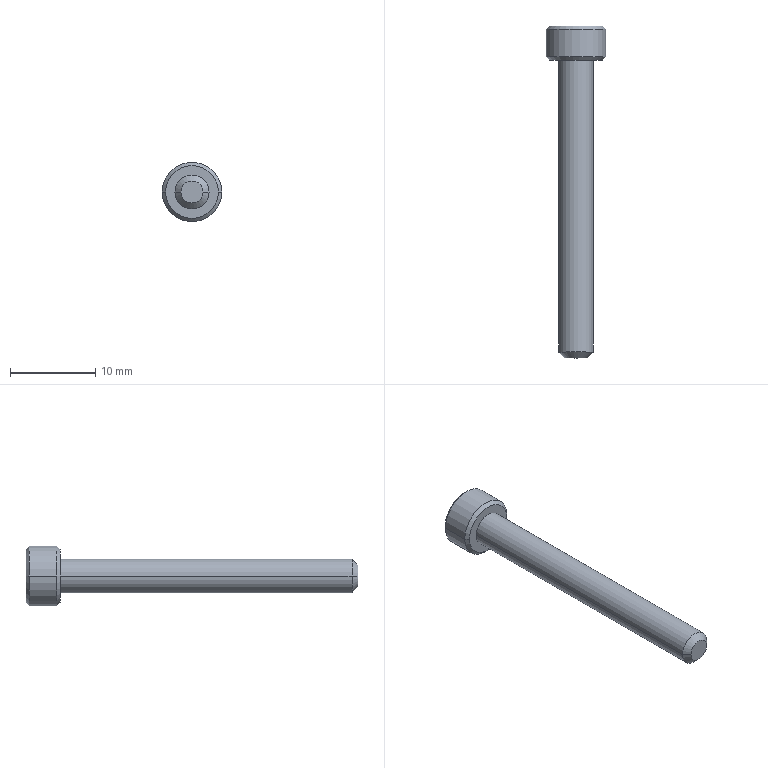Part | STEP file | BB62-M4-35L-16 | 1 solid | 27 faces | box 7 x 39 x 7 mm | volume 569.208 mm3 | plane 15 | cone 8 | cylinder 4 | commonest cylinder face diameters 4 x2 7 x2
STEP:
#1=CARTESIAN_POINT('',(0.,1.007,0.));
#2=VERTEX_POINT('',#1);
#3=CARTESIAN_POINT('',(1.72,2.,0.));
#4=VERTEX_POINT('',#3);
#5=CARTESIAN_POINT('',(0.,1.007,0.));
#6=DIRECTION('',(0.866,0.5,0.));
#7=VECTOR('',#6,1000.);
#8=LINE('',#5,#7);
#9=EDGE_CURVE('',#2,#4,#8,.T.);
#10=ORIENTED_EDGE('',*,*,#9,.F.);
#11=CARTESIAN_POINT('',(-1.72,2.,0.));
#12=VERTEX_POINT('',#11);
#13=CARTESIAN_POINT('',(0.,1.007,0.));
#14=DIRECTION('',(-0.866,0.5,0.));
#15=VECTOR('',#14,1000.);
#16=LINE('',#13,#15);
#17=EDGE_CURVE('',#2,#12,#16,.T.);
#18=ORIENTED_EDGE('',*,*,#17,.T.);
#19=CARTESIAN_POINT('',(-1.49,2.,0.86));
#20=VERTEX_POINT('',#19);
#21=CARTESIAN_POINT('',(0.,2.,0.));
#22=DIRECTION('',(0.,-1.,0.));
#23=DIRECTION('',(-1.,0.,0.));
#24=AXIS2_PLACEMENT_3D('',#21,#22,#23);
#25=CIRCLE('',#24,1.72);
#26=EDGE_CURVE('',#20,#12,#25,.T.);
#27=ORIENTED_EDGE('',*,*,#26,.F.);
#28=CARTESIAN_POINT('',(0.,2.,1.72));
#29=VERTEX_POINT('',#28);
#30=CARTESIAN_POINT('',(0.,2.,0.));
#31=DIRECTION('',(0.,-1.,0.));
#32=DIRECTION('',(-1.,0.,0.));
#33=AXIS2_PLACEMENT_3D('',#30,#31,#32);
#34=CIRCLE('',#33,1.72);
#35=EDGE_CURVE('',#29,#20,#34,.T.);
#36=ORIENTED_EDGE('',*,*,#35,.F.);
#37=CARTESIAN_POINT('',(1.49,2.,0.86));
#38=VERTEX_POINT('',#37);
#39=CARTESIAN_POINT('',(0.,2.,0.));
#40=DIRECTION('',(0.,-1.,0.));
#41=DIRECTION('',(-1.,0.,0.));
#42=AXIS2_PLACEMENT_3D('',#39,#40,#41);
#43=CIRCLE('',#42,1.72);
#44=EDGE_CURVE('',#38,#29,#43,.T.);
#45=ORIENTED_EDGE('',*,*,#44,.F.);
#46=CARTESIAN_POINT('',(0.,2.,0.));
#47=DIRECTION('',(0.,-1.,0.));
#48=DIRECTION('',(-1.,0.,0.));
#49=AXIS2_PLACEMENT_3D('',#46,#47,#48);
#50=CIRCLE('',#49,1.72);
#51=EDGE_CURVE('',#4,#38,#50,.T.);
#52=ORIENTED_EDGE('',*,*,#51,.F.);
#53=EDGE_LOOP('',(#10,#18,#27,#36,#45,#52));
#54=FACE_OUTER_BOUND('',#53,.T.);
#55=CARTESIAN_POINT('',(0.,1001.007,0.));
#56=DIRECTION('',(0.,1.,0.));
#57=DIRECTION('',(1.,0.,0.));
#58=AXIS2_PLACEMENT_3D('',#55,#56,#57);
#59=CONICAL_SURFACE('',#58,1732.051,1.047);
#60=ADVANCED_FACE('',(#54),#59,.F.);
#61=CARTESIAN_POINT('',(1.3,-35.,0.));
#62=VERTEX_POINT('',#61);
#63=CARTESIAN_POINT('',(-1.3,-35.,0.));
#64=VERTEX_POINT('',#63);
#65=CARTESIAN_POINT('',(0.,-35.,0.));
#66=DIRECTION('',(0.,1.,0.));
#67=DIRECTION('',(1.,0.,0.));
#68=AXIS2_PLACEMENT_3D('',#65,#66,#67);
#69=CIRCLE('',#68,1.3);
#70=EDGE_CURVE('',#62,#64,#69,.T.);
#71=ORIENTED_EDGE('',*,*,#70,.T.);
#72=CARTESIAN_POINT('',(-2.,-34.3,0.));
#73=VERTEX_POINT('',#72);
#74=CARTESIAN_POINT('',(-1.3,-35.,0.));
#75=DIRECTION('',(-0.7071,0.7071,0.));
#76=VECTOR('',#75,1000.);
#77=LINE('',#74,#76);
#78=EDGE_CURVE('',#64,#73,#77,.T.);
#79=ORIENTED_EDGE('',*,*,#78,.T.);
#80=CARTESIAN_POINT('',(2.,-34.3,0.));
#81=VERTEX_POINT('',#80);
#82=CARTESIAN_POINT('',(0.,-34.3,0.));
#83=DIRECTION('',(0.,-1.,0.));
#84=DIRECTION('',(-1.,0.,0.));
#85=AXIS2_PLACEMENT_3D('',#82,#83,#84);
#86=CIRCLE('',#85,2.);
#87=EDGE_CURVE('',#73,#81,#86,.T.);
#88=ORIENTED_EDGE('',*,*,#87,.T.);
#89=CARTESIAN_POINT('',(1.3,-35.,0.));
#90=DIRECTION('',(0.7071,0.7071,0.));
#91=VECTOR('',#90,1000.);
#92=LINE('',#89,#91);
#93=EDGE_CURVE('',#62,#81,#92,.T.);
#94=ORIENTED_EDGE('',*,*,#93,.F.);
#95=EDGE_LOOP('',(#71,#79,#88,#94));
#96=FACE_OUTER_BOUND('',#95,.T.);
#97=CARTESIAN_POINT('',(0.,-35.,0.));
#98=DIRECTION('',(0.,1.,0.));
#99=DIRECTION('',(1.,0.,0.));
#100=AXIS2_PLACEMENT_3D('',#97,#98,#99);
#101=CONICAL_SURFACE('',#100,1.3,0.7854);
#102=ADVANCED_FACE('',(#96),#101,.T.);
#103=ORIENTED_EDGE('',*,*,#87,.F.);
#104=CARTESIAN_POINT('',(-2.,0.,0.));
#105=VERTEX_POINT('',#104);
#106=CARTESIAN_POINT('',(-2.,-34.3,0.));
#107=DIRECTION('',(0.,1.,0.));
#108=VECTOR('',#107,1000.);
#109=LINE('',#106,#108);
#110=EDGE_CURVE('',#73,#105,#109,.T.);
#111=ORIENTED_EDGE('',*,*,#110,.T.);
#112=CARTESIAN_POINT('',(2.,0.,0.));
#113=VERTEX_POINT('',#112);
#114=CARTESIAN_POINT('',(0.,0.,0.));
#115=DIRECTION('',(0.,-1.,0.));
#116=DIRECTION('',(-1.,0.,0.));
#117=AXIS2_PLACEMENT_3D('',#114,#115,#116);
#118=CIRCLE('',#117,2.);
#119=EDGE_CURVE('',#105,#113,#118,.T.);
#120=ORIENTED_EDGE('',*,*,#119,.T.);
#121=CARTESIAN_POINT('',(2.,-34.3,0.));
#122=DIRECTION('',(0.,1.,0.));
#123=VECTOR('',#122,1000.);
#124=LINE('',#121,#123);
#125=EDGE_CURVE('',#81,#113,#124,.T.);
#126=ORIENTED_EDGE('',*,*,#125,.F.);
#127=EDGE_LOOP('',(#103,#111,#120,#126));
#128=FACE_OUTER_BOUND('',#127,.T.);
#129=CARTESIAN_POINT('',(0.,-34.3,0.));
#130=DIRECTION('',(0.,1.,0.));
#131=DIRECTION('',(1.,0.,0.));
#132=AXIS2_PLACEMENT_3D('',#129,#130,#131);
#133=CYLINDRICAL_SURFACE('',#132,2.);
#134=ADVANCED_FACE('',(#128),#133,.T.);
#135=CARTESIAN_POINT('',(-3.1,4.,0.));
#136=VERTEX_POINT('',#135);
#137=CARTESIAN_POINT('',(3.1,4.,0.));
#138=VERTEX_POINT('',#137);
#139=CARTESIAN_POINT('',(0.,4.,0.));
#140=DIRECTION('',(0.,-1.,0.));
#141=DIRECTION('',(-1.,0.,0.));
#142=AXIS2_PLACEMENT_3D('',#139,#140,#141);
#143=CIRCLE('',#142,3.1);
#144=EDGE_CURVE('',#136,#138,#143,.T.);
#145=ORIENTED_EDGE('',*,*,#144,.T.);
#146=CARTESIAN_POINT('',(3.5,3.6,0.));
#147=VERTEX_POINT('',#146);
#148=CARTESIAN_POINT('',(3.5,3.6,0.));
#149=DIRECTION('',(0.7071,-0.7071,0.));
#150=VECTOR('',#149,1000.);
#151=LINE('',#148,#150);
#152=EDGE_CURVE('',#138,#147,#151,.T.);
#153=ORIENTED_EDGE('',*,*,#152,.T.);
#154=CARTESIAN_POINT('',(-3.5,3.6,0.));
#155=VERTEX_POINT('',#154);
#156=CARTESIAN_POINT('',(0.,3.6,0.));
#157=DIRECTION('',(0.,-1.,0.));
#158=DIRECTION('',(-1.,0.,0.));
#159=AXIS2_PLACEMENT_3D('',#156,#157,#158);
#160=CIRCLE('',#159,3.5);
#161=EDGE_CURVE('',#155,#147,#160,.T.);
#162=ORIENTED_EDGE('',*,*,#161,.F.);
#163=CARTESIAN_POINT('',(-3.5,3.6,0.));
#164=DIRECTION('',(-0.7071,-0.7071,0.));
#165=VECTOR('',#164,1000.);
#166=LINE('',#163,#165);
#167=EDGE_CURVE('',#136,#155,#166,.T.);
#168=ORIENTED_EDGE('',*,*,#167,.F.);
#169=EDGE_LOOP('',(#145,#153,#162,#168));
#170=FACE_OUTER_BOUND('',#169,.T.);
#171=CARTESIAN_POINT('',(0.,3.6,0.));
#172=DIRECTION('',(0.,-1.,0.));
#173=DIRECTION('',(-1.,0.,0.));
#174=AXIS2_PLACEMENT_3D('',#171,#172,#173);
#175=CONICAL_SURFACE('',#174,3.5,0.7854);
#176=ADVANCED_FACE('',(#170),#175,.T.);
#177=ORIENTED_EDGE('',*,*,#161,.T.);
#178=CARTESIAN_POINT('',(3.5,0.4,0.));
#179=VERTEX_POINT('',#178);
#180=CARTESIAN_POINT('',(3.5,1.62,0.));
#181=DIRECTION('',(0.,-1.,0.));
#182=VECTOR('',#181,1000.);
#183=LINE('',#180,#182);
#184=EDGE_CURVE('',#147,#179,#183,.T.);
#185=ORIENTED_EDGE('',*,*,#184,.T.);
#186=CARTESIAN_POINT('',(-3.5,0.4,0.));
#187=VERTEX_POINT('',#186);
#188=CARTESIAN_POINT('',(0.,0.4,0.));
#189=DIRECTION('',(0.,-1.,0.));
#190=DIRECTION('',(-1.,0.,0.));
#191=AXIS2_PLACEMENT_3D('',#188,#189,#190);
#192=CIRCLE('',#191,3.5);
#193=EDGE_CURVE('',#187,#179,#192,.T.);
#194=ORIENTED_EDGE('',*,*,#193,.F.);
#195=CARTESIAN_POINT('',(-3.5,1.62,0.));
#196=DIRECTION('',(0.,-1.,0.));
#197=VECTOR('',#196,1000.);
#198=LINE('',#195,#197);
#199=EDGE_CURVE('',#155,#187,#198,.T.);
#200=ORIENTED_EDGE('',*,*,#199,.F.);
#201=EDGE_LOOP('',(#177,#185,#194,#200));
#202=FACE_OUTER_BOUND('',#201,.T.);
#203=CARTESIAN_POINT('',(0.,1.62,0.));
#204=DIRECTION('',(0.,-1.,0.));
#205=DIRECTION('',(-1.,0.,0.));
#206=AXIS2_PLACEMENT_3D('',#203,#204,#205);
#207=CYLINDRICAL_SURFACE('',#206,3.5);
#208=ADVANCED_FACE('',(#202),#207,.T.);
#209=CARTESIAN_POINT('',(-3.1,0.,0.));
#210=VERTEX_POINT('',#209);
#211=CARTESIAN_POINT('',(3.1,0.,0.));
#212=VERTEX_POINT('',#211);
#213=CARTESIAN_POINT('',(0.,0.,0.));
#214=DIRECTION('',(0.,-1.,0.));
#215=DIRECTION('',(-1.,0.,0.));
#216=AXIS2_PLACEMENT_3D('',#213,#214,#215);
#217=CIRCLE('',#216,3.1);
#218=EDGE_CURVE('',#210,#212,#217,.T.);
#219=ORIENTED_EDGE('',*,*,#218,.F.);
#220=CARTESIAN_POINT('',(-3.1,0.,0.));
#221=DIRECTION('',(-0.7071,0.7071,0.));
#222=VECTOR('',#221,1000.);
#223=LINE('',#220,#222);
#224=EDGE_CURVE('',#210,#187,#223,.T.);
#225=ORIENTED_EDGE('',*,*,#224,.T.);
#226=ORIENTED_EDGE('',*,*,#193,.T.);
#227=CARTESIAN_POINT('',(3.1,0.,0.));
#228=DIRECTION('',(0.7071,0.7071,0.));
#229=VECTOR('',#228,1000.);
#230=LINE('',#227,#229);
#231=EDGE_CURVE('',#212,#179,#230,.T.);
#232=ORIENTED_EDGE('',*,*,#231,.F.);
#233=EDGE_LOOP('',(#219,#225,#226,#232));
#234=FACE_OUTER_BOUND('',#233,.T.);
#235=CARTESIAN_POINT('',(0.,0.,0.));
#236=DIRECTION('',(0.,1.,0.));
#237=DIRECTION('',(1.,0.,0.));
#238=AXIS2_PLACEMENT_3D('',#235,#236,#237);
#239=CONICAL_SURFACE('',#238,3.1,0.7854);
#240=ADVANCED_FACE('',(#234),#239,.T.);
#241=ORIENTED_EDGE('',*,*,#144,.F.);
#242=CARTESIAN_POINT('',(0.,4.,0.));
#243=DIRECTION('',(0.,-1.,0.));
#244=DIRECTION('',(-1.,0.,0.));
#245=AXIS2_PLACEMENT_3D('',#242,#243,#244);
#246=CIRCLE('',#245,3.1);
#247=EDGE_CURVE('',#138,#136,#246,.T.);
#248=ORIENTED_EDGE('',*,*,#247,.F.);
#249=EDGE_LOOP('',(#241,#248));
#250=FACE_OUTER_BOUND('',#249,.T.);
#251=CARTESIAN_POINT('',(0.,4.,-1.72));
#252=VERTEX_POINT('',#251);
#253=CARTESIAN_POINT('',(-1.49,4.,-0.86));
#254=VERTEX_POINT('',#253);
#255=CARTESIAN_POINT('',(0.,4.,-1.72));
#256=DIRECTION('',(-0.866,0.,0.5));
#257=VECTOR('',#256,1000.);
#258=LINE('',#255,#257);
#259=EDGE_CURVE('',#252,#254,#258,.T.);
#260=ORIENTED_EDGE('',*,*,#259,.F.);
#261=CARTESIAN_POINT('',(1.49,4.,-0.86));
#262=VERTEX_POINT('',#261);
#263=CARTESIAN_POINT('',(1.49,4.,-0.86));
#264=DIRECTION('',(-0.866,0.,-0.5));
#265=VECTOR('',#264,1000.);
#266=LINE('',#263,#265);
#267=EDGE_CURVE('',#262,#252,#266,.T.);
#268=ORIENTED_EDGE('',*,*,#267,.F.);
#269=CARTESIAN_POINT('',(1.49,4.,0.86));
#270=VERTEX_POINT('',#269);
#271=CARTESIAN_POINT('',(1.49,4.,0.86));
#272=DIRECTION('',(0.,0.,-1.));
#273=VECTOR('',#272,1000.);
#274=LINE('',#271,#273);
#275=EDGE_CURVE('',#270,#262,#274,.T.);
#276=ORIENTED_EDGE('',*,*,#275,.F.);
#277=CARTESIAN_POINT('',(0.,4.,1.72));
#278=VERTEX_POINT('',#277);
#279=CARTESIAN_POINT('',(0.,4.,1.72));
#280=DIRECTION('',(0.866,0.,-0.5));
#281=VECTOR('',#280,1000.);
#282=LINE('',#279,#281);
#283=EDGE_CURVE('',#278,#270,#282,.T.);
#284=ORIENTED_EDGE('',*,*,#283,.F.);
#285=CARTESIAN_POINT('',(-1.49,4.,0.86));
#286=VERTEX_POINT('',#285);
#287=CARTESIAN_POINT('',(-1.49,4.,0.86));
#288=DIRECTION('',(0.866,0.,0.5));
#289=VECTOR('',#288,1000.);
#290=LINE('',#287,#289);
#291=EDGE_CURVE('',#286,#278,#290,.T.);
#292=ORIENTED_EDGE('',*,*,#291,.F.);
#293=CARTESIAN_POINT('',(-1.49,4.,-0.86));
#294=DIRECTION('',(0.,0.,1.));
#295=VECTOR('',#294,1000.);
#296=LINE('',#293,#295);
#297=EDGE_CURVE('',#254,#286,#296,.T.);
#298=ORIENTED_EDGE('',*,*,#297,.F.);
#299=EDGE_LOOP('',(#260,#268,#276,#284,#292,#298));
#300=FACE_BOUND('',#299,.T.);
#301=CARTESIAN_POINT('',(3.1,4.,0.));
#302=DIRECTION('',(0.,1.,0.));
#303=DIRECTION('',(1.,0.,0.));
#304=AXIS2_PLACEMENT_3D('',#301,#302,#303);
#305=PLANE('',#304);
#306=ADVANCED_FACE('',(#250,#300),#305,.T.);
#307=CARTESIAN_POINT('',(0.,0.,0.));
#308=DIRECTION('',(0.,-1.,0.));
#309=DIRECTION('',(-1.,0.,0.));
#310=AXIS2_PLACEMENT_3D('',#307,#308,#309);
#311=CIRCLE('',#310,2.);
#312=EDGE_CURVE('',#113,#105,#311,.T.);
#313=ORIENTED_EDGE('',*,*,#312,.F.);
#314=ORIENTED_EDGE('',*,*,#119,.F.);
#315=EDGE_LOOP('',(#313,#314));
#316=FACE_BOUND('',#315,.T.);
#317=CARTESIAN_POINT('',(0.,0.,0.));
#318=DIRECTION('',(0.,-1.,0.));
#319=DIRECTION('',(-1.,0.,0.));
#320=AXIS2_PLACEMENT_3D('',#317,#318,#319);
#321=CIRCLE('',#320,3.1);
#322=EDGE_CURVE('',#212,#210,#321,.T.);
#323=ORIENTED_EDGE('',*,*,#322,.T.);
#324=ORIENTED_EDGE('',*,*,#218,.T.);
#325=EDGE_LOOP('',(#323,#324));
#326=FACE_OUTER_BOUND('',#325,.T.);
#327=CARTESIAN_POINT('',(0.,0.,0.));
#328=DIRECTION('',(0.,-1.,0.));
#329=DIRECTION('',(-1.,0.,0.));
#330=AXIS2_PLACEMENT_3D('',#327,#328,#329);
#331=PLANE('',#330);
#332=ADVANCED_FACE('',(#316,#326),#331,.T.);
#333=ORIENTED_EDGE('',*,*,#224,.F.);
#334=ORIENTED_EDGE('',*,*,#322,.F.);
#335=ORIENTED_EDGE('',*,*,#231,.T.);
#336=CARTESIAN_POINT('',(0.,0.4,0.));
#337=DIRECTION('',(0.,-1.,0.));
#338=DIRECTION('',(-1.,0.,0.));
#339=AXIS2_PLACEMENT_3D('',#336,#337,#338);
#340=CIRCLE('',#339,3.5);
#341=EDGE_CURVE('',#179,#187,#340,.T.);
#342=ORIENTED_EDGE('',*,*,#341,.T.);
#343=EDGE_LOOP('',(#333,#334,#335,#342));
#344=FACE_OUTER_BOUND('',#343,.T.);
#345=CARTESIAN_POINT('',(0.,0.,0.));
#346=DIRECTION('',(0.,1.,0.));
#347=DIRECTION('',(1.,0.,0.));
#348=AXIS2_PLACEMENT_3D('',#345,#346,#347);
#349=CONICAL_SURFACE('',#348,3.1,0.7854);
#350=ADVANCED_FACE('',(#344),#349,.T.);
#351=ORIENTED_EDGE('',*,*,#184,.F.);
#352=CARTESIAN_POINT('',(0.,3.6,0.));
#353=DIRECTION('',(0.,-1.,0.));
#354=DIRECTION('',(-1.,0.,0.));
#355=AXIS2_PLACEMENT_3D('',#352,#353,#354);
#356=CIRCLE('',#355,3.5);
#357=EDGE_CURVE('',#147,#155,#356,.T.);
#358=ORIENTED_EDGE('',*,*,#357,.T.);
#359=ORIENTED_EDGE('',*,*,#199,.T.);
#360=ORIENTED_EDGE('',*,*,#341,.F.);
#361=EDGE_LOOP('',(#351,#358,#359,#360));
#362=FACE_OUTER_BOUND('',#361,.T.);
#363=CARTESIAN_POINT('',(0.,1.62,0.));
#364=DIRECTION('',(0.,-1.,0.));
#365=DIRECTION('',(-1.,0.,0.));
#366=AXIS2_PLACEMENT_3D('',#363,#364,#365);
#367=CYLINDRICAL_SURFACE('',#366,3.5);
#368=ADVANCED_FACE('',(#362),#367,.T.);
#369=ORIENTED_EDGE('',*,*,#152,.F.);
#370=ORIENTED_EDGE('',*,*,#247,.T.);
#371=ORIENTED_EDGE('',*,*,#167,.T.);
#372=ORIENTED_EDGE('',*,*,#357,.F.);
#373=EDGE_LOOP('',(#369,#370,#371,#372));
#374=FACE_OUTER_BOUND('',#373,.T.);
#375=CARTESIAN_POINT('',(0.,3.6,0.));
#376=DIRECTION('',(0.,-1.,0.));
#377=DIRECTION('',(-1.,0.,0.));
#378=AXIS2_PLACEMENT_3D('',#375,#376,#377);
#379=CONICAL_SURFACE('',#378,3.5,0.7854);
#380=ADVANCED_FACE('',(#374),#379,.T.);
#381=ORIENTED_EDGE('',*,*,#110,.F.);
#382=CARTESIAN_POINT('',(0.,-34.3,0.));
#383=DIRECTION('',(0.,-1.,0.));
#384=DIRECTION('',(-1.,0.,0.));
#385=AXIS2_PLACEMENT_3D('',#382,#383,#384);
#386=CIRCLE('',#385,2.);
#387=EDGE_CURVE('',#81,#73,#386,.T.);
#388=ORIENTED_EDGE('',*,*,#387,.F.);
#389=ORIENTED_EDGE('',*,*,#125,.T.);
#390=ORIENTED_EDGE('',*,*,#312,.T.);
#391=EDGE_LOOP('',(#381,#388,#389,#390));
#392=FACE_OUTER_BOUND('',#391,.T.);
#393=CARTESIAN_POINT('',(0.,-34.3,0.));
#394=DIRECTION('',(0.,1.,0.));
#395=DIRECTION('',(1.,0.,0.));
#396=AXIS2_PLACEMENT_3D('',#393,#394,#395);
#397=CYLINDRICAL_SURFACE('',#396,2.);
#398=ADVANCED_FACE('',(#392),#397,.T.);
#399=ORIENTED_EDGE('',*,*,#70,.F.);
#400=CARTESIAN_POINT('',(0.,-35.,0.));
#401=DIRECTION('',(0.,1.,0.));
#402=DIRECTION('',(1.,0.,0.));
#403=AXIS2_PLACEMENT_3D('',#400,#401,#402);
#404=CIRCLE('',#403,1.3);
#405=EDGE_CURVE('',#64,#62,#404,.T.);
#406=ORIENTED_EDGE('',*,*,#405,.F.);
#407=EDGE_LOOP('',(#399,#406));
#408=FACE_OUTER_BOUND('',#407,.T.);
#409=CARTESIAN_POINT('',(0.,-35.,0.));
#410=DIRECTION('',(0.,-1.,0.));
#411=DIRECTION('',(-1.,0.,0.));
#412=AXIS2_PLACEMENT_3D('',#409,#410,#411);
#413=PLANE('',#412);
#414=ADVANCED_FACE('',(#408),#413,.T.);
#415=ORIENTED_EDGE('',*,*,#78,.F.);
#416=ORIENTED_EDGE('',*,*,#405,.T.);
#417=ORIENTED_EDGE('',*,*,#93,.T.);
#418=ORIENTED_EDGE('',*,*,#387,.T.);
#419=EDGE_LOOP('',(#415,#416,#417,#418));
#420=FACE_OUTER_BOUND('',#419,.T.);
#421=CARTESIAN_POINT('',(0.,-35.,0.));
#422=DIRECTION('',(0.,1.,0.));
#423=DIRECTION('',(1.,0.,0.));
#424=AXIS2_PLACEMENT_3D('',#421,#422,#423);
#425=CONICAL_SURFACE('',#424,1.3,0.7854);
#426=ADVANCED_FACE('',(#420),#425,.T.);
#427=CARTESIAN_POINT('',(1.49,2.,-0.86));
#428=VERTEX_POINT('',#427);
#429=CARTESIAN_POINT('',(0.,2.,-1.72));
#430=VERTEX_POINT('',#429);
#431=CARTESIAN_POINT('',(1.49,2.,-0.86));
#432=DIRECTION('',(-0.866,0.,-0.5));
#433=VECTOR('',#432,1000.);
#434=LINE('',#431,#433);
#435=EDGE_CURVE('',#428,#430,#434,.T.);
#436=ORIENTED_EDGE('',*,*,#435,.F.);
#437=CARTESIAN_POINT('',(1.49,4.,-0.86));
#438=DIRECTION('',(0.,-1.,0.));
#439=VECTOR('',#438,1000.);
#440=LINE('',#437,#439);
#441=EDGE_CURVE('',#262,#428,#440,.T.);
#442=ORIENTED_EDGE('',*,*,#441,.F.);
#443=ORIENTED_EDGE('',*,*,#267,.T.);
#444=CARTESIAN_POINT('',(0.,4.,-1.72));
#445=DIRECTION('',(0.,-1.,0.));
#446=VECTOR('',#445,1000.);
#447=LINE('',#444,#446);
#448=EDGE_CURVE('',#252,#430,#447,.T.);
#449=ORIENTED_EDGE('',*,*,#448,.T.);
#450=EDGE_LOOP('',(#436,#442,#443,#449));
#451=FACE_OUTER_BOUND('',#450,.T.);
#452=CARTESIAN_POINT('',(1.49,4.,-0.86));
#453=DIRECTION('',(-0.5,0.,0.866));
#454=DIRECTION('',(0.866,0.,0.5));
#455=AXIS2_PLACEMENT_3D('',#452,#453,#454);
#456=PLANE('',#455);
#457=ADVANCED_FACE('',(#451),#456,.T.);
#458=CARTESIAN_POINT('',(-1.49,2.,-0.86));
#459=VERTEX_POINT('',#458);
#460=CARTESIAN_POINT('',(0.,2.,-1.72));
#461=DIRECTION('',(-0.866,0.,0.5));
#462=VECTOR('',#461,1000.);
#463=LINE('',#460,#462);
#464=EDGE_CURVE('',#430,#459,#463,.T.);
#465=ORIENTED_EDGE('',*,*,#464,.F.);
#466=ORIENTED_EDGE('',*,*,#448,.F.);
#467=ORIENTED_EDGE('',*,*,#259,.T.);
#468=CARTESIAN_POINT('',(-1.49,4.,-0.86));
#469=DIRECTION('',(0.,-1.,0.));
#470=VECTOR('',#469,1000.);
#471=LINE('',#468,#470);
#472=EDGE_CURVE('',#254,#459,#471,.T.);
#473=ORIENTED_EDGE('',*,*,#472,.T.);
#474=EDGE_LOOP('',(#465,#466,#467,#473));
#475=FACE_OUTER_BOUND('',#474,.T.);
#476=CARTESIAN_POINT('',(0.,4.,-1.72));
#477=DIRECTION('',(0.5,0.,0.866));
#478=DIRECTION('',(0.866,0.,-0.5));
#479=AXIS2_PLACEMENT_3D('',#476,#477,#478);
#480=PLANE('',#479);
#481=ADVANCED_FACE('',(#475),#480,.T.);
#482=CARTESIAN_POINT('',(-1.49,2.,-0.86));
#483=DIRECTION('',(0.,0.,1.));
#484=VECTOR('',#483,1000.);
#485=LINE('',#482,#484);
#486=EDGE_CURVE('',#459,#20,#485,.T.);
#487=ORIENTED_EDGE('',*,*,#486,.F.);
#488=ORIENTED_EDGE('',*,*,#472,.F.);
#489=ORIENTED_EDGE('',*,*,#297,.T.);
#490=CARTESIAN_POINT('',(-1.49,4.,0.86));
#491=DIRECTION('',(0.,-1.,0.));
#492=VECTOR('',#491,1000.);
#493=LINE('',#490,#492);
#494=EDGE_CURVE('',#286,#20,#493,.T.);
#495=ORIENTED_EDGE('',*,*,#494,.T.);
#496=EDGE_LOOP('',(#487,#488,#489,#495));
#497=FACE_OUTER_BOUND('',#496,.T.);
#498=CARTESIAN_POINT('',(-1.49,4.,-0.86));
#499=DIRECTION('',(1.,0.,0.));
#500=DIRECTION('',(0.,0.,-1.));
#501=AXIS2_PLACEMENT_3D('',#498,#499,#500);
#502=PLANE('',#501);
#503=ADVANCED_FACE('',(#497),#502,.T.);
#504=CARTESIAN_POINT('',(-1.49,2.,0.86));
#505=DIRECTION('',(0.866,0.,0.5));
#506=VECTOR('',#505,1000.);
#507=LINE('',#504,#506);
#508=EDGE_CURVE('',#20,#29,#507,.T.);
#509=ORIENTED_EDGE('',*,*,#508,.F.);
#510=ORIENTED_EDGE('',*,*,#494,.F.);
#511=ORIENTED_EDGE('',*,*,#291,.T.);
#512=CARTESIAN_POINT('',(0.,4.,1.72));
#513=DIRECTION('',(0.,-1.,0.));
#514=VECTOR('',#513,1000.);
#515=LINE('',#512,#514);
#516=EDGE_CURVE('',#278,#29,#515,.T.);
#517=ORIENTED_EDGE('',*,*,#516,.T.);
#518=EDGE_LOOP('',(#509,#510,#511,#517));
#519=FACE_OUTER_BOUND('',#518,.T.);
#520=CARTESIAN_POINT('',(-1.49,4.,0.86));
#521=DIRECTION('',(0.5,0.,-0.866));
#522=DIRECTION('',(-0.866,0.,-0.5));
#523=AXIS2_PLACEMENT_3D('',#520,#521,#522);
#524=PLANE('',#523);
#525=ADVANCED_FACE('',(#519),#524,.T.);
#526=CARTESIAN_POINT('',(0.,2.,1.72));
#527=DIRECTION('',(0.866,0.,-0.5));
#528=VECTOR('',#527,1000.);
#529=LINE('',#526,#528);
#530=EDGE_CURVE('',#29,#38,#529,.T.);
#531=ORIENTED_EDGE('',*,*,#530,.F.);
#532=ORIENTED_EDGE('',*,*,#516,.F.);
#533=ORIENTED_EDGE('',*,*,#283,.T.);
#534=CARTESIAN_POINT('',(1.49,4.,0.86));
#535=DIRECTION('',(0.,-1.,0.));
#536=VECTOR('',#535,1000.);
#537=LINE('',#534,#536);
#538=EDGE_CURVE('',#270,#38,#537,.T.);
#539=ORIENTED_EDGE('',*,*,#538,.T.);
#540=EDGE_LOOP('',(#531,#532,#533,#539));
#541=FACE_OUTER_BOUND('',#540,.T.);
#542=CARTESIAN_POINT('',(0.,4.,1.72));
#543=DIRECTION('',(-0.5,0.,-0.866));
#544=DIRECTION('',(-0.866,0.,0.5));
#545=AXIS2_PLACEMENT_3D('',#542,#543,#544);
#546=PLANE('',#545);
#547=ADVANCED_FACE('',(#541),#546,.T.);
#548=CARTESIAN_POINT('',(1.49,2.,0.86));
#549=DIRECTION('',(0.,0.,-1.));
#550=VECTOR('',#549,1000.);
#551=LINE('',#548,#550);
#552=EDGE_CURVE('',#38,#428,#551,.T.);
#553=ORIENTED_EDGE('',*,*,#552,.F.);
#554=ORIENTED_EDGE('',*,*,#538,.F.);
#555=ORIENTED_EDGE('',*,*,#275,.T.);
#556=ORIENTED_EDGE('',*,*,#441,.T.);
#557=EDGE_LOOP('',(#553,#554,#555,#556));
#558=FACE_OUTER_BOUND('',#557,.T.);
#559=CARTESIAN_POINT('',(1.49,4.,0.86));
#560=DIRECTION('',(-1.,0.,0.));
#561=DIRECTION('',(0.,0.,1.));
#562=AXIS2_PLACEMENT_3D('',#559,#560,#561);
#563=PLANE('',#562);
#564=ADVANCED_FACE('',(#558),#563,.T.);
#565=ORIENTED_EDGE('',*,*,#435,.T.);
#566=CARTESIAN_POINT('',(0.,2.,0.));
#567=DIRECTION('',(0.,-1.,0.));
#568=DIRECTION('',(-1.,0.,0.));
#569=AXIS2_PLACEMENT_3D('',#566,#567,#568);
#570=CIRCLE('',#569,1.72);
#571=EDGE_CURVE('',#430,#428,#570,.T.);
#572=ORIENTED_EDGE('',*,*,#571,.T.);
#573=EDGE_LOOP('',(#565,#572));
#574=FACE_OUTER_BOUND('',#573,.T.);
#575=CARTESIAN_POINT('',(0.,2.,0.));
#576=DIRECTION('',(0.,1.,0.));
#577=DIRECTION('',(1.,0.,0.));
#578=AXIS2_PLACEMENT_3D('',#575,#576,#577);
#579=PLANE('',#578);
#580=ADVANCED_FACE('',(#574),#579,.F.);
#581=ORIENTED_EDGE('',*,*,#552,.T.);
#582=CARTESIAN_POINT('',(0.,2.,0.));
#583=DIRECTION('',(0.,-1.,0.));
#584=DIRECTION('',(-1.,0.,0.));
#585=AXIS2_PLACEMENT_3D('',#582,#583,#584);
#586=CIRCLE('',#585,1.72);
#587=EDGE_CURVE('',#428,#4,#586,.T.);
#588=ORIENTED_EDGE('',*,*,#587,.T.);
#589=ORIENTED_EDGE('',*,*,#51,.T.);
#590=EDGE_LOOP('',(#581,#588,#589));
#591=FACE_OUTER_BOUND('',#590,.T.);
#592=CARTESIAN_POINT('',(0.,2.,0.));
#593=DIRECTION('',(0.,1.,0.));
#594=DIRECTION('',(1.,0.,0.));
#595=AXIS2_PLACEMENT_3D('',#592,#593,#594);
#596=PLANE('',#595);
#597=ADVANCED_FACE('',(#591),#596,.F.);
#598=ORIENTED_EDGE('',*,*,#530,.T.);
#599=ORIENTED_EDGE('',*,*,#44,.T.);
#600=EDGE_LOOP('',(#598,#599));
#601=FACE_OUTER_BOUND('',#600,.T.);
#602=CARTESIAN_POINT('',(0.,2.,0.));
#603=DIRECTION('',(0.,1.,0.));
#604=DIRECTION('',(1.,0.,0.));
#605=AXIS2_PLACEMENT_3D('',#602,#603,#604);
#606=PLANE('',#605);
#607=ADVANCED_FACE('',(#601),#606,.F.);
#608=ORIENTED_EDGE('',*,*,#508,.T.);
#609=ORIENTED_EDGE('',*,*,#35,.T.);
#610=EDGE_LOOP('',(#608,#609));
#611=FACE_OUTER_BOUND('',#610,.T.);
#612=CARTESIAN_POINT('',(0.,2.,0.));
#613=DIRECTION('',(0.,1.,0.));
#614=DIRECTION('',(1.,0.,0.));
#615=AXIS2_PLACEMENT_3D('',#612,#613,#614);
#616=PLANE('',#615);
#617=ADVANCED_FACE('',(#611),#616,.F.);
#618=ORIENTED_EDGE('',*,*,#486,.T.);
#619=ORIENTED_EDGE('',*,*,#26,.T.);
#620=CARTESIAN_POINT('',(0.,2.,0.));
#621=DIRECTION('',(0.,-1.,0.));
#622=DIRECTION('',(-1.,0.,0.));
#623=AXIS2_PLACEMENT_3D('',#620,#621,#622);
#624=CIRCLE('',#623,1.72);
#625=EDGE_CURVE('',#12,#459,#624,.T.);
#626=ORIENTED_EDGE('',*,*,#625,.T.);
#627=EDGE_LOOP('',(#618,#619,#626));
#628=FACE_OUTER_BOUND('',#627,.T.);
#629=CARTESIAN_POINT('',(0.,2.,0.));
#630=DIRECTION('',(0.,1.,0.));
#631=DIRECTION('',(1.,0.,0.));
#632=AXIS2_PLACEMENT_3D('',#629,#630,#631);
#633=PLANE('',#632);
#634=ADVANCED_FACE('',(#628),#633,.F.);
#635=ORIENTED_EDGE('',*,*,#464,.T.);
#636=CARTESIAN_POINT('',(0.,2.,0.));
#637=DIRECTION('',(0.,-1.,0.));
#638=DIRECTION('',(-1.,0.,0.));
#639=AXIS2_PLACEMENT_3D('',#636,#637,#638);
#640=CIRCLE('',#639,1.72);
#641=EDGE_CURVE('',#459,#430,#640,.T.);
#642=ORIENTED_EDGE('',*,*,#641,.T.);
#643=EDGE_LOOP('',(#635,#642));
#644=FACE_OUTER_BOUND('',#643,.T.);
#645=CARTESIAN_POINT('',(0.,2.,0.));
#646=DIRECTION('',(0.,1.,0.));
#647=DIRECTION('',(1.,0.,0.));
#648=AXIS2_PLACEMENT_3D('',#645,#646,#647);
#649=PLANE('',#648);
#650=ADVANCED_FACE('',(#644),#649,.F.);
#651=ORIENTED_EDGE('',*,*,#17,.F.);
#652=ORIENTED_EDGE('',*,*,#9,.T.);
#653=ORIENTED_EDGE('',*,*,#587,.F.);
#654=ORIENTED_EDGE('',*,*,#571,.F.);
#655=ORIENTED_EDGE('',*,*,#641,.F.);
#656=ORIENTED_EDGE('',*,*,#625,.F.);
#657=EDGE_LOOP('',(#651,#652,#653,#654,#655,#656));
#658=FACE_OUTER_BOUND('',#657,.T.);
#659=CARTESIAN_POINT('',(0.,1001.007,0.));
#660=DIRECTION('',(0.,1.,0.));
#661=DIRECTION('',(1.,0.,0.));
#662=AXIS2_PLACEMENT_3D('',#659,#660,#661);
#663=CONICAL_SURFACE('',#662,1732.051,1.047);
#664=ADVANCED_FACE('',(#658),#663,.F.);
#665=CLOSED_SHELL('',(#60,#102,#134,#176,#208,#240,#306,#332,#350,#368,#380,#398,#414,#426,#457,#481,#503,#525,#547,#564,#580,#597,#607,#617,#634,#650,#664));
#666=MANIFOLD_SOLID_BREP('',#665);
#667=CARTESIAN_POINT('',(0.,0.,0.));
#668=DIRECTION('',(0.,0.,1.));
#669=DIRECTION('',(1.,0.,0.));
#670=AXIS2_PLACEMENT_3D('',#667,#668,#669);
#671=(LENGTH_UNIT()NAMED_UNIT(*)SI_UNIT(.MILLI.,.METRE.));
#672=UNCERTAINTY_MEASURE_WITH_UNIT(LENGTH_MEASURE(0.00001),#671,'','');
#673=(NAMED_UNIT(*)PLANE_ANGLE_UNIT()SI_UNIT($,.RADIAN.));
#674=(NAMED_UNIT(*)SI_UNIT($,.STERADIAN.)SOLID_ANGLE_UNIT());
#675=(GEOMETRIC_REPRESENTATION_CONTEXT(3)GLOBAL_UNCERTAINTY_ASSIGNED_CONTEXT((#672))GLOBAL_UNIT_ASSIGNED_CONTEXT((#671,#673,#674))REPRESENTATION_CONTEXT('',''));
#676=ADVANCED_BREP_SHAPE_REPRESENTATION('',(#666,#670),#675);